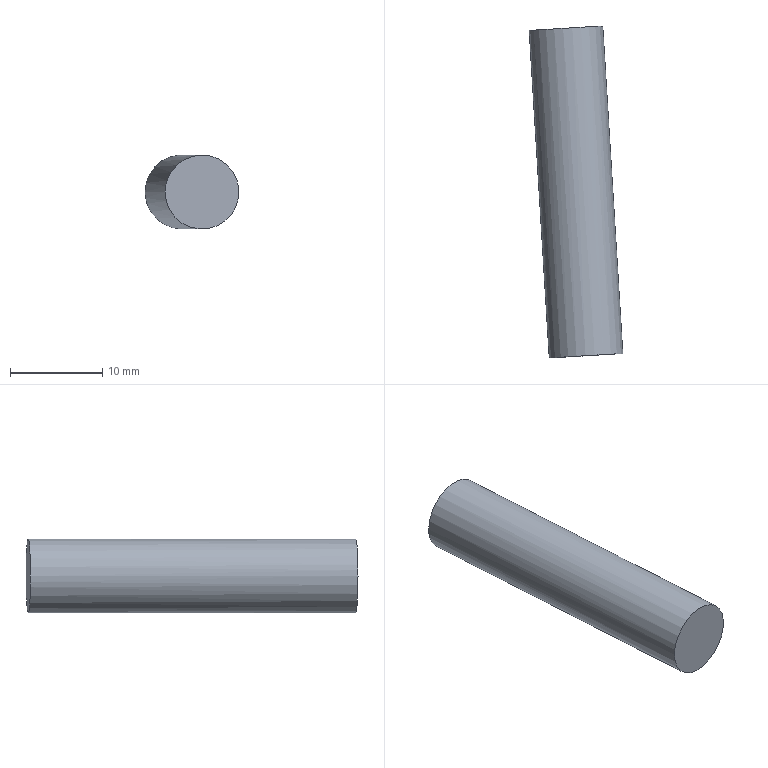Part | STEP file | 车灯-后视镜_id342_x_t | 1 solid | 3 faces | box 10.152 x 35.922 x 8 mm | volume 1784 mm3 | plane 2 | cylinder 1 | commonest cylinder face diameters 8 x1
STEP:
#1=CARTESIAN_POINT('',(93.445,28.049,-237.501));
#2=VERTEX_POINT('',#1);
#3=CARTESIAN_POINT('',(97.437,28.293,-237.501));
#4=DIRECTION('',(-0.061,0.9981,0.));
#5=DIRECTION('',(-0.9981,-0.061,0.));
#6=AXIS2_PLACEMENT_3D('',#3,#4,#5);
#7=ELLIPSE('',#6,4.,4.);
#8=EDGE_CURVE('',#2,#2,#7,.T.);
#9=ORIENTED_EDGE('',*,*,#8,.T.);
#10=EDGE_LOOP('',(#9));
#11=FACE_OUTER_BOUND('',#10,.T.);
#12=CARTESIAN_POINT('',(66.345,26.392,3.882));
#13=DIRECTION('',(0.061,-0.9981,0.));
#14=DIRECTION('',(0.9981,0.061,0.));
#15=AXIS2_PLACEMENT_3D('',#12,#13,#14);
#16=PLANE('',#15);
#17=ADVANCED_FACE('',(#11),#16,.F.);
#18=CARTESIAN_POINT('',(95.612,-7.385,-237.501));
#19=VERTEX_POINT('',#18);
#20=CARTESIAN_POINT('',(99.604,-7.141,-237.501));
#21=DIRECTION('',(0.061,-0.9981,0.));
#22=DIRECTION('',(-0.9981,-0.061,0.));
#23=AXIS2_PLACEMENT_3D('',#20,#21,#22);
#24=ELLIPSE('',#23,4.,4.);
#25=EDGE_CURVE('',#19,#19,#24,.T.);
#26=ORIENTED_EDGE('',*,*,#25,.F.);
#27=EDGE_LOOP('',(#26));
#28=FACE_BOUND('',#27,.T.);
#29=ORIENTED_EDGE('',*,*,#8,.F.);
#30=EDGE_LOOP('',(#29));
#31=FACE_BOUND('',#30,.T.);
#32=CARTESIAN_POINT('',(99.696,-8.639,-237.501));
#33=DIRECTION('',(-0.06105,0.9981,0.));
#34=DIRECTION('',(-0.9981,-0.06105,0.));
#35=AXIS2_PLACEMENT_3D('',#32,#33,#34);
#36=CYLINDRICAL_SURFACE('',#35,4.);
#37=ADVANCED_FACE('',(#28,#31),#36,.T.);
#38=ORIENTED_EDGE('',*,*,#25,.T.);
#39=EDGE_LOOP('',(#38));
#40=FACE_OUTER_BOUND('',#39,.T.);
#41=CARTESIAN_POINT('',(68.51,-9.042,3.882));
#42=DIRECTION('',(0.061,-0.9981,0.));
#43=DIRECTION('',(0.9981,0.061,0.));
#44=AXIS2_PLACEMENT_3D('',#41,#42,#43);
#45=PLANE('',#44);
#46=ADVANCED_FACE('',(#40),#45,.T.);
#47=CLOSED_SHELL('',(#17,#37,#46));
#48=MANIFOLD_SOLID_BREP('',#47);
#49=(LENGTH_UNIT()NAMED_UNIT(*)SI_UNIT(.MILLI.,.METRE.));
#50=UNCERTAINTY_MEASURE_WITH_UNIT(LENGTH_MEASURE(0.00002),#49,'','');
#51=(NAMED_UNIT(*)PLANE_ANGLE_UNIT()SI_UNIT($,.RADIAN.));
#52=PLANE_ANGLE_MEASURE_WITH_UNIT(PLANE_ANGLE_MEASURE(0.01745),#51);
#53=DIMENSIONAL_EXPONENTS(0.,0.,0.,0.,0.,0.,0.);
#54=(CONVERSION_BASED_UNIT('DEGREE',#52)NAMED_UNIT(#53)PLANE_ANGLE_UNIT());
#55=(NAMED_UNIT(*)SI_UNIT($,.STERADIAN.)SOLID_ANGLE_UNIT());
#56=(GEOMETRIC_REPRESENTATION_CONTEXT(3)GLOBAL_UNCERTAINTY_ASSIGNED_CONTEXT((#50))GLOBAL_UNIT_ASSIGNED_CONTEXT((#49,#54,#55))REPRESENTATION_CONTEXT('',''));
#57=ADVANCED_BREP_SHAPE_REPRESENTATION('',(#48),#56);